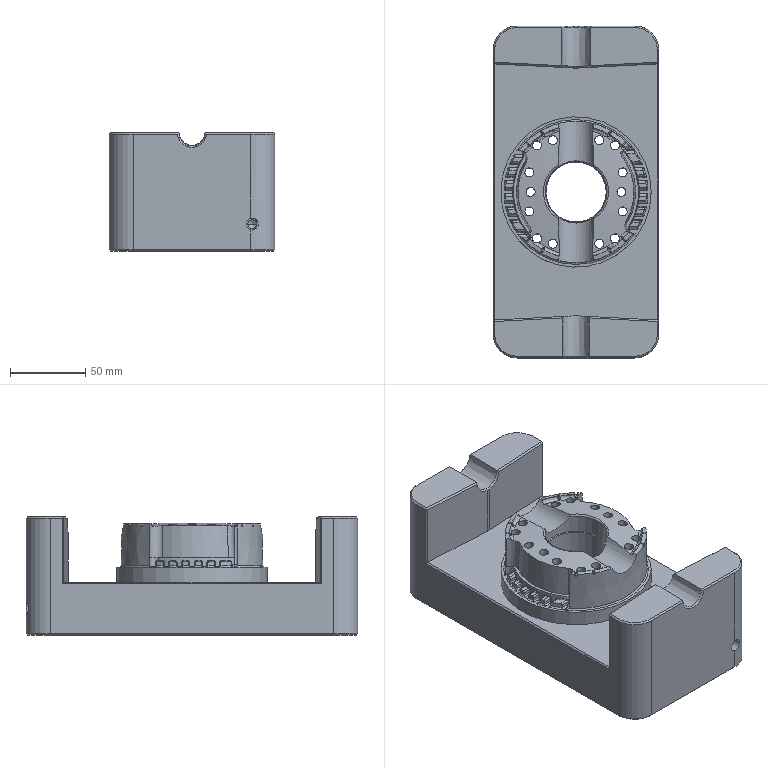Part | NX | features solid 2 | 1 solid | 458 faces | box 110 x 220 x 78.508 mm | volume 1161319 mm3 | cylinder 176 | plane 122 | spline 75 | torus 50 | cone 21 | sphere 14 | commonest cylinder face diameters 2.01 x53 1.005 x36 6 x25 93.465 x12 88.038 x11 8 x9